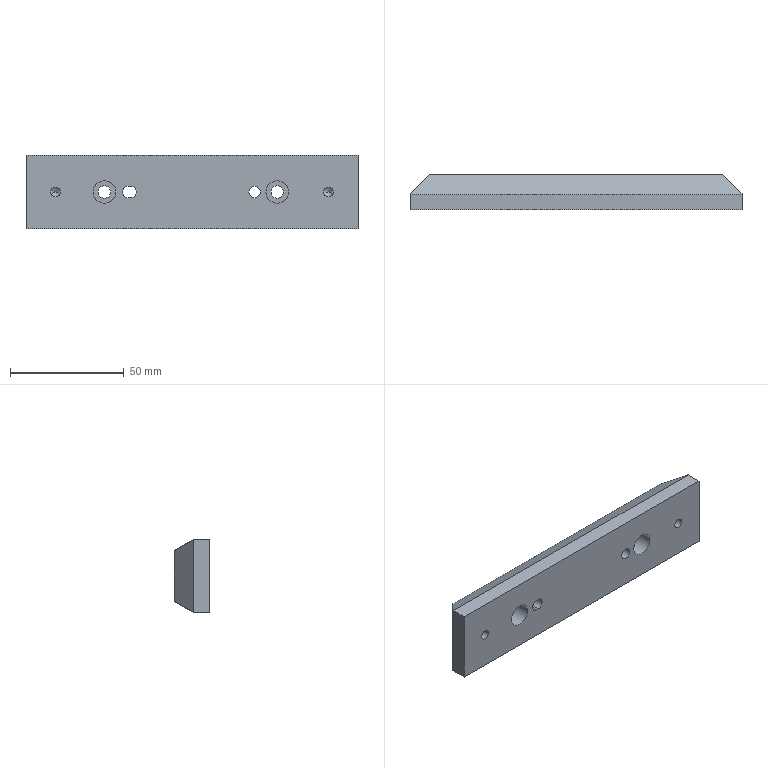NC program | NX | posted with a generic post | part box 146 x 15.5 x 32.5 mm
Lines 1 to 1077 of 14263:
N10 G17 G21 G94 G90
(ZLEVEL_PROFILE_COPY_1 , TOOL : D6R0.5)
N12 T16 M6
N14 G54
N16 G17 G0 G90 X7.285 Y-29.91 S9500 M3
N18 G43 Z30. H16
N20 Z1.5
N22 G94 G1 X7.11 Y-29.829 Z1.49 F1000.
N24 X6.592 Y-29.424 Z1.455
N26 X6.178 Y-28.913 Z1.421
N28 X5.89 Y-28.322 Z1.387
N30 X5.743 Y-27.681 Z1.352
N32 X5.735 Y-27.441 Z1.339
N34 Y-27.097 Z1.321
N36 Y-5.403 Z0.185
N38 Y-5.059 Z0.166
N40 X5.743 Y-4.819 Z0.154
N42 X5.89 Y-4.178 Z0.119
N44 X6.178 Y-3.587 Z0.085
N46 X6.592 Y-3.076 Z0.05
N48 X7.11 Y-2.671 Z0.016
N50 X7.706 Y-2.394 Z-0.018
N52 X8.35 Y-2.257 Z-0.053
N54 X8.59 Y-2.255 Z-0.065
N56 X137.41 Y-2.254 F3000.
N58 G2 X140.265 Y-5.059 R2.891
N60 G1 Y-5.403
N62 Y-27.097
N64 Y-27.441
N66 G2 X137.41 Y-30.245 R2.89
N68 G1 X8.59 Y-30.246
N70 G2 X5.735 Y-27.441 R2.891
N72 G1 Y-27.097
N74 Y-5.403
N76 Y-5.059
N78 G2 X8.59 Y-2.255 R2.89
N80 G1 X14.446 Y-2.25 Z-0.067
N82 X134.482 Y-2.236 Z-0.091
N84 X137.41 Y-2.239 Z-0.092
N86 X137.631 Y-2.252
N88 X137.852 Y-2.276
N90 X138.069 Y-2.324
N92 X138.285 Y-2.378
N94 X138.492 Y-2.459
N96 X138.698 Y-2.545
N98 X138.891 Y-2.656
N100 X139.08 Y-2.775
N102 X139.256 Y-2.912
N104 X139.424 Y-3.059
N106 X139.577 Y-3.222
N108 X139.72 Y-3.394
N110 X139.846 Y-3.579
N112 X139.96 Y-3.771
N114 X140.055 Y-3.974 Z-0.093
N116 X140.138 Y-4.182
N118 X140.2 Y-4.396
N120 X140.249 Y-4.614
N122 X140.277 Y-4.836
N124 X140.292 Y-5.059
N126 X140.293 Y-5.403
N128 Y-8.115
N130 X140.297 Y-27.269 Z-0.097
N132 Y-27.441
N134 X140.281 Y-27.665
N136 X140.254 Y-27.886
N138 X140.205 Y-28.105
N140 X140.143 Y-28.32 Z-0.098
N142 X140.061 Y-28.528
N144 X139.965 Y-28.731
N146 X139.851 Y-28.924
N148 X139.725 Y-29.11
N150 X139.582 Y-29.282
N152 X139.428 Y-29.445
N154 X139.26 Y-29.592
N156 X139.083 Y-29.73
N158 X138.894 Y-29.849
N160 X138.7 Y-29.96
N162 X138.494 Y-30.046
N164 X138.286 Y-30.127
N166 X138.07 Y-30.181
N168 X137.853 Y-30.228
N170 X137.632 Y-30.252
N172 X137.41 Y-30.265
N174 X131.554 Y-30.269 Z-0.099
N176 X11.518 Y-30.283 Z-0.124
N178 X8.59 Y-30.281 Z-0.125
N180 X8.367 Y-30.269
N182 X8.144 Y-30.248
N184 X7.925 Y-30.201
N186 X7.707 Y-30.149
N188 X7.497 Y-30.068
N190 X7.288 Y-29.984
N192 X7.092 Y-29.872
N194 X6.9 Y-29.754
N196 X6.721 Y-29.615
N198 X6.551 Y-29.467
N200 X6.395 Y-29.302
N202 X6.25 Y-29.129
N204 X6.122 Y-28.941
N206 X6.007 Y-28.746
N208 X5.91 Y-28.541
N210 X5.827 Y-28.33
N212 X5.765 Y-28.113
N214 X5.716 Y-27.892
N216 X5.689 Y-27.667
N218 X5.675 Y-27.442 Z-0.126
N220 X5.674 Y-27.269
N222 X5.671 Y-8.115 Z-0.129
N224 X5.67 Y-5.403 Z-0.13
N226 Y-5.231
N228 Y-5.058
N230 X5.684 Y-4.832
N232 X5.711 Y-4.607
N234 X5.76 Y-4.386
N236 X5.821 Y-4.168
N238 X5.905 Y-3.957
N240 X6.001 Y-3.751
N242 X6.117 Y-3.556
N244 X6.245 Y-3.368
N246 X6.39 Y-3.194 Z-0.131
N248 X6.546 Y-3.029
N250 X6.718 Y-2.88
N252 X6.897 Y-2.741
N254 X7.089 Y-2.623
N256 X7.286 Y-2.511
N258 X7.495 Y-2.427
N260 X7.705 Y-2.347
N262 X7.924 Y-2.294
N264 X8.144 Y-2.248
N266 X8.367 Y-2.227
N268 X8.59 Y-2.215
N270 X11.518 Y-2.213 Z-0.132
N272 X134.482 Y-2.198 Z-0.157
N274 X137.41 Y-2.199
N276 X137.582 Y-2.205
N278 X137.753 Y-2.215
N280 X137.863 Y-2.229
N282 X138.085 Y-2.275
N284 X138.307 Y-2.327 Z-0.158
N286 X138.52 Y-2.406
N288 X138.732 Y-2.491
N290 X138.931 Y-2.603
N292 X139.125 Y-2.722
N294 X139.306 Y-2.862
N296 X139.479 Y-3.011
N298 X139.637 Y-3.177
N300 X139.784 Y-3.353
N302 X139.912 Y-3.542
N304 X140.029 Y-3.739
N306 X140.126 Y-3.947
N308 X140.209 Y-4.16
N310 X140.271 Y-4.38
N312 X140.319 Y-4.604
N314 X140.345 Y-4.826
N316 X140.358 Y-5.049
N318 X140.359 Y-7.852 Z-0.159
N320 X140.362 Y-24.648 Z-0.162
N322 X140.363 Y-27.451 Z-0.163
N324 X140.35 Y-27.674
N326 X140.324 Y-27.897
N328 X140.276 Y-28.121
N330 X140.215 Y-28.342
N332 X140.131 Y-28.555
N334 X140.034 Y-28.763
N336 X139.917 Y-28.961
N338 X139.788 Y-29.151
N340 X139.641 Y-29.327
N342 X139.483 Y-29.493
N344 X139.31 Y-29.643
N346 X139.129 Y-29.783
N348 X138.934 Y-29.902
N350 X138.734 Y-30.014
N352 X138.522 Y-30.099 Z-0.164
N354 X138.308 Y-30.178
N356 X138.087 Y-30.23
N358 X137.863 Y-30.276
N360 X137.754 Y-30.289
N362 X137.582 Y-30.299
N364 X137.41 Y-30.305
N366 X131.554 Y-30.307 Z-0.165
N368 X46.651 Y-30.317 Z-0.182
N370 X43.723 Y-30.316 Z-0.183
N372 X40.795 Y-30.317 Z-0.184
N374 X37.867
N376 X34.94 Y-30.318 Z-0.185
N378 X32.012
N380 X29.084 Y-30.319 Z-0.186
N382 X26.157
N384 X23.229 Z-0.187
N386 X11.518 Y-30.321 Z-0.189
N388 X8.59 Z-0.19
N390 X8.417 Y-30.316
N392 X8.244 Y-30.305
N394 X8.135 Y-30.294
N396 X7.909 Y-30.25
N398 X7.685 Y-30.2
N400 X7.469 Y-30.121
N402 X7.255 Y-30.037
N404 X7.053 Y-29.925
N406 X6.855 Y-29.806
N408 X6.671 Y-29.666 Z-0.191
N410 X6.496 Y-29.515
N412 X6.336 Y-29.347
N414 X6.187 Y-29.17
N416 X6.056 Y-28.978
N418 X5.938 Y-28.778
N420 X5.84 Y-28.568
N422 X5.756 Y-28.352
N424 X5.694 Y-28.128
N426 X5.646 Y-27.902
N428 X5.621 Y-27.677
N430 X5.609 Y-27.451
N432 X5.604 Y-5.048 Z-0.196
N434 X5.616 Y-4.822
N436 X5.641 Y-4.598
N438 X5.689 Y-4.37
N440 X5.75 Y-4.147
N442 X5.835 Y-3.93
N444 X5.933 Y-3.719
N446 X6.051 Y-3.519
N448 X6.182 Y-3.327
N450 X6.331 Y-3.149
N452 X6.492 Y-2.981
N454 X6.668 Y-2.83
N456 X6.851 Y-2.689
N458 X7.05 Y-2.57
N460 X7.253 Y-2.458
N462 X7.467 Y-2.374
N464 X7.684 Y-2.295
N466 X7.908 Y-2.245
N468 X8.134 Y-2.202
N470 X8.244 Y-2.191
N472 X8.416 Y-2.181 Z-0.197
N474 X8.589 Y-2.176
N476 X14.446 Y-2.175 Z-0.198
N478 X137.41 Y-2.16 Z-0.223
N480 X137.487 Y-2.162
N482 X137.622 Y-2.166
N484 X137.757 Y-2.172
N486 X137.994 Y-2.201
N488 X138.228 Y-2.249
N490 X138.458 Y-2.316
N492 X138.682 Y-2.401
N494 X138.897 Y-2.504
N496 X139.104 Y-2.626
N498 X139.299 Y-2.764
N500 X139.392 Y-2.84
N502 X139.484 Y-2.917
N504 X139.569 Y-3.001
N506 X139.655 Y-3.085
N508 X139.733 Y-3.175
N510 X139.812 Y-3.267
N512 X139.882 Y-3.364
N514 X139.952 Y-3.461
N516 X140.014 Y-3.564
N518 X140.076 Y-3.667
N520 X140.129 Y-3.775 Z-0.224
N522 X140.182 Y-3.882
N524 X140.226 Y-3.994
N526 X140.269 Y-4.106
N528 X140.304 Y-4.221
N530 X140.337 Y-4.336
N532 X140.362 Y-4.454
N534 X140.386 Y-4.571
N536 X140.41 Y-4.791
N538 X140.424 Y-5.048
N540 X140.428 Y-27.489 Z-0.228
N542 X140.415 Y-27.71
N544 X140.391 Y-27.93
N546 X140.367 Y-28.047
N548 X140.342 Y-28.165
N550 X140.309 Y-28.28 Z-0.229
N552 X140.275 Y-28.396
N554 X140.231 Y-28.508
N556 X140.187 Y-28.62
N558 X140.134 Y-28.728
N560 X140.081 Y-28.836
N562 X140.019 Y-28.939
N564 X139.957 Y-29.042
N566 X139.887 Y-29.14
N568 X139.816 Y-29.237
N570 X139.738 Y-29.329
N572 X139.659 Y-29.42
N574 X139.574 Y-29.504
N576 X139.488 Y-29.588
N578 X139.395 Y-29.664
N580 X139.303 Y-29.741
N582 X139.107 Y-29.879
N584 X138.9 Y-30.001
N586 X138.684 Y-30.104
N588 X138.459 Y-30.189
N590 X138.229 Y-30.255
N592 X137.995 Y-30.304
N594 X137.758 Y-30.333
N596 X137.622 Y-30.338
N598 X137.487 Y-30.342
N600 X137.41 Y-30.344
N602 X8.512 Y-30.359 Z-0.256
N604 X8.376
N606 X8.241 Y-30.35
N608 X8.002 Y-30.322
N610 X7.766 Y-30.275
N612 X7.534 Y-30.21
N614 X7.307 Y-30.126
N616 X7.088 Y-30.024
N618 X6.879 Y-29.902
N620 X6.68 Y-29.763
N622 X6.586 Y-29.687
N624 X6.492 Y-29.61
N626 X6.405 Y-29.525
N628 X6.318 Y-29.44
N630 X6.238 Y-29.349
N632 X6.159 Y-29.257
N634 X6.087 Y-29.158
N636 X6.016 Y-29.06
N638 X5.953 Y-28.956
N640 X5.891 Y-28.851
N642 X5.837 Y-28.742
N644 X5.784 Y-28.633
N646 X5.739 Y-28.52
N648 X5.696 Y-28.406
N650 X5.661 Y-28.289
N652 X5.628 Y-28.173
N654 X5.603 Y-28.054
N656 X5.58 Y-27.935
N658 X5.556 Y-27.712 Z-0.257
N660 X5.543 Y-27.452
N662 X5.539 Y-5.011 Z-0.261
N664 X5.551 Y-4.787
N666 X5.575 Y-4.565
N668 X5.598 Y-4.445
N670 X5.622 Y-4.326
N672 X5.656 Y-4.209
N674 X5.69 Y-4.092
N676 X5.734 Y-3.978
N678 X5.778 Y-3.865
N680 X5.832 Y-3.755
N682 X5.886 Y-3.646
N684 X5.948 Y-3.541
N686 X6.011 Y-3.437
N688 X6.082 Y-3.338
N690 X6.154 Y-3.24 Z-0.262
N692 X6.234 Y-3.147
N694 X6.314 Y-3.056
N696 X6.401 Y-2.97
N698 X6.488 Y-2.886
N700 X6.582 Y-2.808
N702 X6.676 Y-2.732
N704 X6.876 Y-2.593
N706 X7.085 Y-2.471
N708 X7.305 Y-2.369
N710 X7.532 Y-2.285
N712 X7.765 Y-2.221
N714 X8.001 Y-2.174
N716 X8.241 Y-2.146
N718 X8.376 Y-2.137
N720 X8.589
N722 X137.529 Y-2.122 Z-0.288
N724 X137.571
N726 X137.666
N728 X137.761
N730 X137.855 Y-2.135
N732 X137.949 Y-2.147
N734 X138.176 Y-2.191 Z-0.289
N736 X138.402 Y-2.241
N738 X138.62 Y-2.319
N740 X138.835 Y-2.405
N742 X139.04 Y-2.515
N744 X139.238 Y-2.635
N746 X139.424 Y-2.775
N748 X139.6 Y-2.926
N750 X139.761 Y-3.095
N752 X139.911 Y-3.273
N754 X140.042 Y-3.465
N756 X140.161 Y-3.666
N758 X140.18 Y-3.702
N760 X140.267 Y-3.896
N762 X140.344 Y-4.095
N764 X140.376 Y-4.207
N766 X140.408 Y-4.32
N768 X140.454 Y-4.548
N770 X140.475 Y-4.74
N772 X140.488 Y-4.933
N774 X140.489 Y-4.972
N776 X140.494 Y-27.527 Z-0.294
N778 X140.481 Y-27.74
N780 X140.458 Y-27.953
N782 X140.411 Y-28.182
N784 X140.349 Y-28.407
N786 X140.265 Y-28.625
N788 X140.167 Y-28.837
N790 X140.048 Y-29.038
N792 X139.916 Y-29.231
N794 X139.766 Y-29.41
N796 X139.604 Y-29.578
N798 X139.427 Y-29.73
N800 X139.241 Y-29.87
N802 X139.042 Y-29.99 Z-0.295
N804 X138.837 Y-30.1
N806 X138.641 Y-30.179
N808 X138.403 Y-30.262
N810 X138.177 Y-30.314
N812 X137.95 Y-30.358
N814 X137.855 Y-30.369
N816 X137.761 Y-30.382
N818 X137.571
N820 X137.529
N822 X8.429 Y-30.397 Z-0.321
N824 X8.238
N826 X8.048 Y-30.375
N828 X7.819 Y-30.334
N830 X7.591 Y-30.284
N832 X7.37 Y-30.208
N834 X7.153 Y-30.121
N836 X6.944 Y-30.013
N838 X6.743 Y-29.892 Z-0.322
N840 X6.554 Y-29.752
N842 X6.375 Y-29.6
N844 X6.211 Y-29.43
N846 X6.059 Y-29.25
N848 X5.926 Y-29.055
N850 X5.806 Y-28.852
N852 X5.786 Y-28.815
N854 X5.698 Y-28.618
N856 X5.617 Y-28.418
N858 X5.552 Y-28.19
N860 X5.507 Y-27.958
N862 X5.491 Y-27.763
N864 X5.478 Y-27.568
N866 X5.473 Y-4.973 Z-0.327
N868 X5.485 Y-4.757
N870 X5.506 Y-4.541
N872 X5.554 Y-4.31
N874 X5.616 Y-4.082
N876 X5.701 Y-3.861
N878 X5.8 Y-3.646
N880 X5.921 Y-3.442
N882 X6.054 Y-3.246
N884 X6.207 Y-3.066
N886 X6.371 Y-2.895
N888 X6.551 Y-2.743
N890 X6.74 Y-2.602
N892 X6.942 Y-2.481
N894 X7.151 Y-2.374
N896 X7.348 Y-2.294
N898 X7.59 Y-2.215
N900 X7.817 Y-2.162
N902 X8.048 Y-2.122 Z-0.328
N904 X8.238 Y-2.1
N906 X8.429
N908 X8.589
N910 X137.571 Y-2.084 Z-0.354
N912 X137.636
N914 X137.736
N916 X137.837
N918 X137.936 Y-2.099
N920 X138.035 Y-2.112
N922 X138.264 Y-2.158
N924 X138.491 Y-2.212
N926 X138.711 Y-2.291
N928 X138.927 Y-2.382
N930 X139.133 Y-2.493
N932 X139.331 Y-2.617
N934 X139.517 Y-2.76
N936 X139.693 Y-2.915
N938 X139.853 Y-3.087
N940 X140.002 Y-3.268
N942 X140.068 Y-3.363 Z-0.355
N944 X140.161 Y-3.514
N946 X140.249 Y-3.667
N948 X140.337 Y-3.868
N950 X140.419 Y-4.07
N952 X140.472 Y-4.283
N954 X140.522 Y-4.496
N956 X140.54 Y-4.695
N958 X140.555 Y-4.895
N960 Y-4.932
N962 X140.559 Y-27.565 Z-0.359
N964 X140.547 Y-27.779 Z-0.36
N966 X140.524 Y-27.993
N968 X140.476 Y-28.221
N970 X140.414 Y-28.447
N972 X140.329 Y-28.665
N974 X140.231 Y-28.877
N976 X140.111 Y-29.078
N978 X139.979 Y-29.272
N980 X139.829 Y-29.451
N982 X139.667 Y-29.619
N984 X139.489 Y-29.771
N986 X139.301 Y-29.911
N988 X139.101 Y-30.032
N990 X138.894 Y-30.14
N992 X138.678 Y-30.227
N994 X138.456 Y-30.301
N996 X138.238 Y-30.353
N998 X138.017 Y-30.392
N1000 X137.828 Y-30.419
N1002 X137.636
N1004 X137.603
N1006 X8.364 Y-30.435 Z-0.387
N1008 X8.162
N1010 X7.962 Y-30.41
N1012 X7.73 Y-30.367
N1014 X7.501 Y-30.314
N1016 X7.278 Y-30.236
N1018 X7.06 Y-30.146
N1020 X6.851 Y-30.036
N1022 X6.649 Y-29.911
N1024 X6.46 Y-29.767
N1026 X6.282 Y-29.611
N1028 X6.119 Y-29.438
N1030 X5.968 Y-29.254
N1032 X5.901 Y-29.159
N1034 X5.807 Y-29.006
N1036 X5.716 Y-28.851
N1038 X5.629 Y-28.647
N1040 X5.545 Y-28.441
N1042 X5.493 Y-28.225 Z-0.388
N1044 X5.443 Y-28.009
N1046 X5.426 Y-27.808
N1048 X5.412 Y-27.605
N1050 X5.408 Y-4.935 Z-0.392
N1052 X5.419 Y-4.718
N1054 X5.44 Y-4.502
N1056 X5.489 Y-4.27
N1058 X5.551 Y-4.042
N1060 X5.636 Y-3.82
N1062 X5.736 Y-3.605 Z-0.393
N1064 X5.857 Y-3.401
N1066 X5.991 Y-3.206
N1068 X6.144 Y-3.025
N1070 X6.309 Y-2.854
N1072 X6.49 Y-2.701
N1074 X6.68 Y-2.561
N1076 X6.883 Y-2.44
N1078 X7.094 Y-2.333
N1080 X7.319 Y-2.243
N1082 X7.55 Y-2.17
N1084 X7.763 Y-2.121
N1086 X7.98 Y-2.086
N1088 X8.171 Y-2.062
N1090 X8.364
N1092 X8.589
N1094 X137.669 Y-2.046 Z-0.419
N1096 X137.701 Y-2.047
N1098 X137.806 Z-0.42
N1100 X137.911 Y-2.046
N1102 X138.015 Y-2.063
N1104 X138.119 Y-2.078
N1106 X138.357 Y-2.122
N1108 X138.591 Y-2.186
N1110 X138.82 Y-2.268
N1112 X139.042 Y-2.368
N1114 X139.254 Y-2.486
N1116 X139.457 Y-2.622
N1118 X139.647 Y-2.774
N1120 X139.824 Y-2.942
N1122 X139.985 Y-3.124
N1124 X140.058 Y-3.222
N1126 X140.16 Y-3.362
N1128 X140.252 Y-3.521
N1130 X140.343 Y-3.68
N1132 X140.497 Y-4.07
N1134 X140.591 Y-4.478
N1136 X140.62 Y-4.85
N1138 Y-4.894
N1140 X140.625 Y-27.603 Z-0.425
N1142 X140.612 Y-27.821
N1144 X140.589 Y-28.039
N1146 X140.541 Y-28.272
N1148 X140.474 Y-28.501
N1150 X140.389 Y-28.723
N1152 X140.337 Y-28.83
N1154 X140.284 Y-28.938
N1156 X140.224 Y-29.04
N1158 X140.163 Y-29.143
N1160 X140.094 Y-29.24
N1162 X140.024 Y-29.337
N1164 X139.87 Y-29.518
N1166 X139.701 Y-29.686
N1168 X139.518 Y-29.84 Z-0.426
N1170 X139.324 Y-29.977
N1172 X139.119 Y-30.098
N1174 X138.905 Y-30.202
N1176 X138.684 Y-30.289
N1178 X138.564 Y-30.326
N1180 X138.443 Y-30.36
N1182 X138.247 Y-30.402
N1184 X138.049 Y-30.434
N1186 X137.876 Y-30.457
N1188 X137.701
N1190 X8.298 Y-30.472 Z-0.452
N1192 X8.087
N1194 X7.878 Y-30.445
N1196 X7.637 Y-30.403
N1198 X7.519 Y-30.37
N1200 X7.401 Y-30.34
N1202 X7.169 Y-30.259
N1204 X6.945 Y-30.16 Z-0.453
N1206 X6.729 Y-30.042
N1208 X6.523 Y-29.906
N1210 X6.33 Y-29.753
N1212 X6.15 Y-29.584
N1214 X6.068 Y-29.492
N1216 X5.986 Y-29.4
N1218 X5.912 Y-29.301
N1220 X5.809 Y-29.159
N1222 X5.715 Y-28.998
N1224 X5.622 Y-28.836
N1226 X5.468 Y-28.441
N1228 X5.375 Y-28.027
N1230 X5.347 Y-27.651
N1232 X5.342 Y-4.897 Z-0.458
N1234 X5.358 Y-4.676
N1236 X5.376 Y-4.456
N1238 X5.424 Y-4.219
N1240 X5.491 Y-3.987
N1242 X5.534 Y-3.875
N1244 X5.577 Y-3.762
N1246 X5.629 Y-3.653
N1248 X5.682 Y-3.544
N1250 X5.744 Y-3.44
N1252 X5.806 Y-3.337
N1254 X5.876 Y-3.238
N1256 X5.946 Y-3.14
N1258 X6.025 Y-3.049
N1260 X6.103 Y-2.957
N1262 X6.275 Y-2.787
N1264 X6.46 Y-2.633
N1266 X6.658 Y-2.495
N1268 X6.866 Y-2.374
N1270 X7.083 Y-2.271
N1272 X7.308 Y-2.186 Z-0.459
N1274 X7.55 Y-2.116
N1276 X7.748 Y-2.074
N1278 X7.948 Y-2.045
N1280 X8.123 Y-2.024
N1282 X8.298
N1284 X8.589
N1286 X137.734 Y-2.009 Z-0.485
N1288 X137.767
N1290 X137.945
N1292 X138.122 Y-2.031
N1294 X138.33 Y-2.068
N1296 X138.536 Y-2.113
N1298 X138.738 Y-2.177
N1300 X138.936 Y-2.251
N1302 X139.313 Y-2.444
N1304 X139.487 Y-2.565
N1306 X139.656 Y-2.693
N1308 X139.814 Y-2.834
N1310 X139.963 Y-2.985 Z-0.486
N1312 X140.097 Y-3.149
N1314 X140.222 Y-3.32
N1316 X140.249 Y-3.361
N1318 X140.336 Y-3.517
N1320 X140.423 Y-3.672
N1322 X140.495 Y-3.862
N1324 X140.567 Y-4.051
N1326 X140.611 Y-4.249
N1328 X140.653 Y-4.446
N1330 X140.686 Y-4.817
N1332 Y-4.849
N1334 X140.69 Y-27.64 Z-0.491
N1336 X140.676 Y-27.836
N1338 X140.661 Y-28.032
N1340 X140.618 Y-28.243
N1342 X140.567 Y-28.452
N1344 X140.495 Y-28.655
N1346 X140.412 Y-28.854
N1348 X140.309 Y-29.044
N1350 X140.197 Y-29.228
N1352 X140.066 Y-29.4
N1354 X139.927 Y-29.564
N1356 X139.772 Y-29.714
N1358 X139.61 Y-29.856
N1360 X139.433 Y-29.979
N1362 X139.254 Y-30.098
N1364 X138.866 Y-30.283
N1366 X138.787 Y-30.313
N1368 X138.622 Y-30.365
N1370 X138.456 Y-30.411
N1372 X138.269 Y-30.448
N1374 X138.081 Y-30.476
N1376 X137.924 Y-30.495
N1378 X137.767 Z-0.492
N1380 X8.233 Y-30.51 Z-0.518
N1382 X8.053
N1384 X7.875 Y-30.491
N1386 X7.665 Y-30.456
N1388 X7.457 Y-30.413
N1390 X7.253 Y-30.35
N1392 X7.053 Y-30.276
N1394 X6.67 Y-30.084
N1396 X6.493 Y-29.963
N1398 X6.321 Y-29.835
N1400 X6.161 Y-29.692
N1402 X6.01 Y-29.54
N1404 X5.874 Y-29.374
N1406 X5.747 Y-29.2
N1408 X5.72 Y-29.159
N1410 X5.631 Y-29.002
N1412 X5.544 Y-28.844
N1414 X5.47 Y-28.652 Z-0.519
N1416 X5.398 Y-28.46
N1418 X5.354 Y-28.259
N1420 X5.312 Y-28.059
N1422 X5.281 Y-27.683
N1424 X5.277 Y-4.859 Z-0.523
N1426 X5.29 Y-4.661
N1428 X5.304 Y-4.463
N1430 X5.347 Y-4.249
N1432 X5.397 Y-4.037 Z-0.524
N1434 X5.471 Y-3.831
N1436 X5.554 Y-3.63
N1438 X5.658 Y-3.437
N1440 X5.772 Y-3.251
N1442 X5.904 Y-3.077
N1444 X6.047 Y-2.911
N1446 X6.204 Y-2.76
N1448 X6.369 Y-2.617
N1450 X6.548 Y-2.493
N1452 X6.73 Y-2.374
N1454 X7.124 Y-2.19
N1456 X7.204 Y-2.161
N1458 X7.37 Y-2.108
N1460 X7.539 Y-2.066
N1462 X7.727 Y-2.029
N1464 X7.917 Y-2.004
N1466 X8.074 Y-1.986
N1468 X8.233
N1470 X8.589
N1472 X137.767 Y-1.971 Z-0.551
N1474 X137.833
N1476 X138.014
N1478 X138.104 Y-1.983
N1480 X138.194 Y-1.994
N1482 X138.405 Y-2.032
N1484 X138.614 Y-2.078
N1486 X138.818 Y-2.144
N1488 X139.019 Y-2.221
N1490 X139.209 Y-2.321
N1492 X139.398 Y-2.423
N1494 X139.576 Y-2.544
N1496 X139.746 Y-2.675
N1498 X139.905 Y-2.821
N1500 X140.054 Y-2.976
N1502 X140.188 Y-3.145
N1504 X140.312 Y-3.321
N1506 X140.409 Y-3.492
N1508 X140.516 Y-3.699
N1510 X140.639 Y-4.038
N1512 X140.681 Y-4.231
N1514 X140.721 Y-4.424
N1516 X140.751 Y-4.817
N1518 X140.756 Y-27.679 Z-0.556
N1520 X140.741 Y-27.883
N1522 X140.724 Y-28.086
N1524 X140.678 Y-28.305
N1526 X140.622 Y-28.522
N1528 X140.545 Y-28.732
N1530 X140.455 Y-28.937
N1532 X140.345 Y-29.132
N1534 X140.224 Y-29.321
N1536 X140.084 Y-29.496 Z-0.557
N1538 X139.934 Y-29.662
N1540 X139.8 Y-29.786
N1542 X139.659 Y-29.903
N1544 X139.627 Y-29.928
N1546 X139.593 Y-29.952
N1548 X139.407 Y-30.075
N1550 X139.217 Y-30.192
N1552 X139.014 Y-30.286
N1554 X138.806 Y-30.367
N1556 X138.637 Y-30.418
N1558 X138.466 Y-30.462
N1560 X138.292 Y-30.492
N1562 X138.118 Y-30.516
N1564 X137.976 Y-30.533
N1566 X137.8
N1568 X8.167 Y-30.548 Z-0.583
N1570 X7.985
N1572 X7.803 Y-30.528
N1574 X7.59 Y-30.492
N1576 X7.379 Y-30.449 Z-0.584
N1578 X7.172 Y-30.383
N1580 X6.969 Y-30.307
N1582 X6.776 Y-30.207
N1584 X6.584 Y-30.106
N1586 X6.404 Y-29.984
N1588 X6.231 Y-29.852
N1590 X6.07 Y-29.705
N1592 X5.918 Y-29.549
N1594 X5.782 Y-29.378
N1596 X5.657 Y-29.2
N1598 X5.558 Y-29.026
N1600 X5.452 Y-28.816
N1602 X5.388 Y-28.644
N1604 X5.329 Y-28.471
N1606 X5.284 Y-28.277
N1608 X5.245 Y-28.081
N1610 X5.23 Y-27.882
N1612 X5.216 Y-27.683
N1614 X5.211 Y-4.821 Z-0.589
N1616 X5.225 Y-4.615
N1618 X5.241 Y-4.409
N1620 X5.287 Y-4.187
N1622 X5.343 Y-3.967
N1624 X5.421 Y-3.754
N1626 X5.511 Y-3.546
N1628 X5.623 Y-3.348
N1630 X5.746 Y-3.157
N1632 X5.888 Y-2.98
N1634 X6.041 Y-2.812
N1636 X6.177 Y-2.687
N1638 X6.319 Y-2.57
N1640 X6.352 Y-2.544
N1642 X6.386 Y-2.52
N1644 X6.576 Y-2.397
N1646 X6.769 Y-2.281 Z-0.59
N1648 X6.974 Y-2.187
N1650 X7.186 Y-2.107
N1652 X7.356 Y-2.056
N1654 X7.529 Y-2.016
N1656 X7.704 Y-1.984
N1658 X7.88 Y-1.962
N1660 X8.023 Y-1.948
N1662 X8.2
N1664 X8.589
N1666 X137.833 Y-1.933 Z-0.616
N1668 X137.898
N1670 X138.261 Y-1.956
N1672 X138.472 Y-1.995
N1674 X138.682 Y-2.038
N1676 X138.886 Y-2.107
N1678 X139.087 Y-2.183
N1680 X139.467 Y-2.385
N1682 X139.644 Y-2.508
N1684 X139.815 Y-2.64 Z-0.617
N1686 X139.973 Y-2.786
N1688 X140.123 Y-2.942
N1690 X140.257 Y-3.111
N1692 X140.38 Y-3.288
N1694 X140.486 Y-3.476
N1696 X140.581 Y-3.67
N1698 X140.651 Y-3.854
N1700 X140.711 Y-4.042
N1702 X140.755 Y-4.234
N1704 X140.79 Y-4.428
N1706 X140.804 Y-4.606
N1708 X140.817 Y-4.784
N1710 X140.822 Y-27.716 Z-0.622
N1712 X140.807 Y-27.916
N1714 X140.789 Y-28.115
N1716 X140.746 Y-28.33
N1718 X140.693 Y-28.543
N1720 X140.619 Y-28.749
N1722 X140.533 Y-28.951
N1724 X140.427 Y-29.143
N1726 X140.31 Y-29.329
N1728 X140.176 Y-29.502
N1730 X140.031 Y-29.668
N1732 X139.871 Y-29.818
N1734 X139.702 Y-29.958
N1736 X139.537 Y-30.073
N1738 X139.366 Y-30.179
N1740 X139.186 Y-30.267
N1742 X139.006 Y-30.356
N1744 X138.817 Y-30.421
N1746 X138.624 Y-30.479
N1748 X138.428 Y-30.518
N1750 X138.231 Y-30.551 Z-0.623
N1752 X137.898 Y-30.571
N1754 X8.102 Y-30.586 Z-0.649
N1756 X7.737 Y-30.566
N1758 X7.524 Y-30.53
N1760 X7.311 Y-30.487
N1762 X7.105 Y-30.42
N1764 X6.9 Y-30.346
N1766 X6.515 Y-30.144
N1768 X6.335 Y-30.02
N1770 X6.162 Y-29.888
N1772 X6.001 Y-29.74
N1774 X5.849 Y-29.583
N1776 X5.713 Y-29.411
N1778 X5.588 Y-29.232
N1780 X5.48 Y-29.042
N1782 X5.384 Y-28.845 Z-0.65
N1784 X5.314 Y-28.658
N1786 X5.254 Y-28.468
N1788 X5.21 Y-28.273
N1790 X5.177 Y-28.076
N1792 X5.162 Y-27.896
N1794 X5.15 Y-27.716
N1796 X5.146 Y-4.783 Z-0.654
N1798 X5.159 Y-4.581
N1800 X5.178 Y-4.38 Z-0.655
N1802 X5.218 Y-4.161
N1804 X5.272 Y-3.946
N1806 X5.347 Y-3.737
N1808 X5.434 Y-3.533
N1810 X5.541 Y-3.338
N1812 X5.659 Y-3.15
N1814 X5.796 Y-2.974
N1816 X5.943 Y-2.807
N1818 X6.105 Y-2.655
N1820 X6.277 Y-2.514
N1822 X6.444 Y-2.399
N1824 X6.617 Y-2.292
N1826 X6.982 Y-2.114
N1828 X7.175 Y-2.052
N1830 X7.369 Y-1.995
N1832 X7.568 Y-1.958
N1834 X7.767 Y-1.927
N1836 X8.102 Y-1.91
N1838 X8.589
N1840 X137.898 Y-1.895 Z-0.682
N1842 X137.964
N1844 X138.357 Y-1.924
N1846 X138.583 Y-1.967
N1848 X138.808 Y-2.017
N1850 X139.025 Y-2.096
N1852 X139.239 Y-2.183
N1854 X139.439 Y-2.299
N1856 X139.638 Y-2.417
N1858 X139.823 Y-2.556
N1860 X139.998 Y-2.707
N1862 X140.159 Y-2.874
N1864 X140.309 Y-3.052
N1866 X140.439 Y-3.244
N1868 X140.557 Y-3.444
N1870 X140.654 Y-3.655
N1872 X140.737 Y-3.872
N1874 X140.798 Y-4.095
N1876 X140.843 Y-4.323
N1878 X140.866 Y-4.534
N1880 X140.883 Y-4.747 Z-0.683
N1882 X140.887 Y-27.754 Z-0.687
N1884 X140.871 Y-27.966
N1886 X140.848 Y-28.178
N1888 X140.803 Y-28.406
N1890 X140.743 Y-28.63
N1892 X140.66 Y-28.847
N1894 X140.563 Y-29.059
N1896 X140.444 Y-29.259
N1898 X140.314 Y-29.452 Z-0.688
N1900 X140.164 Y-29.63
N1902 X140.003 Y-29.798
N1904 X139.826 Y-29.948
N1906 X139.641 Y-30.088
N1908 X139.442 Y-30.206
N1910 X139.241 Y-30.322
N1912 X139.027 Y-30.409
N1914 X138.81 Y-30.488
N1916 X138.584 Y-30.538
N1918 X138.358 Y-30.58
N1920 X138.161 Y-30.594
N1922 X137.964 Y-30.609
N1924 X137.898
N1926 X8.036 Y-30.624 Z-0.714
N1928 X7.838 Y-30.611
N1930 X7.64 Y-30.597
N1932 X7.411 Y-30.558
N1934 X7.185 Y-30.508 Z-0.715
N1936 X6.964 Y-30.431
N1938 X6.748 Y-30.345
N1940 X6.545 Y-30.23
N1942 X6.343 Y-30.112
N1944 X6.155 Y-29.971
N1946 X5.976 Y-29.819
N1948 X5.813 Y-29.65
N1950 X5.661 Y-29.471
N1952 X5.529 Y-29.276
N1954 X5.409 Y-29.074
N1956 X5.311 Y-28.86
N1958 X5.228 Y-28.64
N1960 X5.167 Y-28.413
N1962 X5.122 Y-28.183
N1964 X5.1 Y-27.969
N1966 X5.085 Y-27.754
N1968 X5.08 Y-4.746 Z-0.72
N1970 X5.095 Y-4.531
N1972 X5.117 Y-4.316
N1974 X5.162 Y-4.085
N1976 X5.222 Y-3.858
N1978 X5.306 Y-3.638
N1980 X5.404 Y-3.424
N1982 X5.524 Y-3.22
N1984 X5.656 Y-3.025
N1986 X5.808 Y-2.846
N1988 X5.972 Y-2.676
N1990 X6.151 Y-2.524
N1992 X6.339 Y-2.383
N1994 X6.542 Y-2.265 Z-0.721
N1996 X6.745 Y-2.15
N1998 X6.963 Y-2.064
N2000 X7.183 Y-1.987
N2002 X7.41 Y-1.937
N2004 X7.64 Y-1.899
N2006 X7.838 Y-1.885
N2008 X8.036 Y-1.872
N2010 X8.589
N2012 X137.964 Y-1.857 Z-0.747
N2014 X138.029
N2016 X138.423 Y-1.887
N2018 X138.649 Y-1.929
N2020 X138.874 Y-1.98
N2022 X139.091 Y-2.059
N2024 X139.304 Y-2.145
N2026 X139.505 Y-2.261
N2028 X139.703 Y-2.379
N2030 X139.888 Y-2.518 Z-0.748
N2032 X140.064 Y-2.669
N2034 X140.225 Y-2.836
N2036 X140.374 Y-3.014
N2038 X140.505 Y-3.206
N2040 X140.623 Y-3.406
N2042 X140.72 Y-3.617
N2044 X140.803 Y-3.834
N2046 X140.863 Y-4.058
N2048 X140.909 Y-4.285
N2050 X140.932 Y-4.497
N2052 X140.948 Y-4.709
N2054 X140.953 Y-27.791 Z-0.753
N2056 X140.937 Y-28.004
N2058 X140.914 Y-28.216
N2060 X140.869 Y-28.444
N2062 X140.808 Y-28.668
N2064 X140.725 Y-28.885
N2066 X140.628 Y-29.097
N2068 X140.51 Y-29.297
N2070 X140.379 Y-29.49
N2072 X140.229 Y-29.668
N2074 X140.068 Y-29.835
N2076 X139.892 Y-29.986
N2078 X139.707 Y-30.126
N2080 X139.508 Y-30.244
N2082 X139.307 Y-30.36
N2084 X139.093 Y-30.447
N2086 X138.875 Y-30.525
N2088 X138.65 Y-30.576
N2090 X138.423 Y-30.618 Z-0.754
N2092 X138.226 Y-30.632
N2094 X138.029 Y-30.647
N2096 X137.964 Y-30.646
N2098 X8.003 Y-30.662 Z-0.78
N2100 X7.971
N2102 X7.773 Y-30.649
N2104 X7.575 Y-30.635
N2106 X7.346 Y-30.596
N2108 X7.119 Y-30.546
N2110 X6.899 Y-30.469
N2112 X6.682 Y-30.383
N2114 X6.479 Y-30.267
N2116 X6.277 Y-30.15
N2118 X6.09 Y-30.009
N2120 X5.911 Y-29.857
N2122 X5.748 Y-29.688
N2124 X5.596 Y-29.509
N2126 X5.463 Y-29.314
N2128 X5.344 Y-29.111 Z-0.781
N2130 X5.246 Y-28.898
N2132 X5.162 Y-28.678
N2134 X5.101 Y-28.451
N2136 X5.056 Y-28.221
N2138 X5.034 Y-28.007
N2140 X5.019 Y-27.792
N2142 X5.015 Y-4.708 Z-0.785
N2144 X5.029 Y-4.493
N2146 X5.051 Y-4.278 Z-0.786
N2148 X5.096 Y-4.048
N2150 X5.157 Y-3.821
N2152 X5.24 Y-3.6